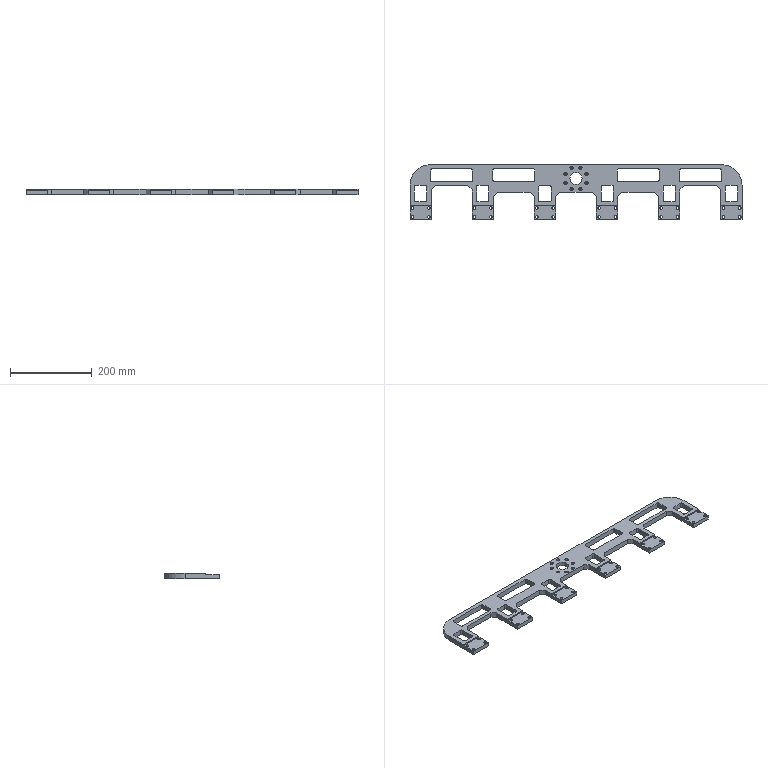NC program | NX | posted with a generic post | part box 813.6 x 134 x 13 mm
Lines 1 to 121 of 13853:
N10 G17 G21 G94 G90
(FLOOR_WALL_COPY , TOOL : D63)
N12 T01 M6
N14 G54
N16 G17 G0 G90 X-443.3 Y68.997 S6500 M3
N18 G43 Z30. H1
N20 Z3.
N22 G94 G1 Z0. F1500.
N24 X-440.3
N26 X440.3
N28 Y40.798
N30 X-440.3
N32 Y12.599
N34 X440.3
N36 Y-15.601
N38 X-440.3
N40 Y-43.8
N42 X440.3
N44 X443.3
N46 Z3.
N48 G0 Z30.
N50 M5
(DRILLING_COPY_1 , TOOL : D6A45)
N52 T07 M6
N54 G54
N56 G17 G0 G90 X-400.8 Y-61.2 S5000 M3
N58 G43 Z30. H7
N60 G94 G81 G98 Z-1. F250. R3.
N62 Y-39.2
N64 X-360.8
N66 Y-61.2
N68 X-248.4 Y-39.2
N70 Y-61.2
N72 X-208.4
N74 Y-39.2
N76 X-96.
N78 Y-61.2
N80 X-56.
N82 Y-39.2
N84 X-10.715 Y7.131
N86 X-25.869 Y22.285
N88 Y43.715
N90 X-10.715 Y58.869
N92 X10.715
N94 X25.869 Y43.715
N96 X0. Y33.
N98 X25.869 Y22.285
N100 X10.715 Y7.131
N102 X56.4 Y-39.2
N104 Y-61.2
N106 X96.4
N108 Y-39.2
N110 X208.8
N112 Y-61.2
N114 X248.8
N116 Y-39.2
N118 X361.2
N120 Y-61.2
N122 X401.2
N124 Y-39.2
N126 G80
N128 G0 X401.2 Y-39.2 Z30.
N130 M5
(DRILLING_COPY_COPY_1 , TOOL : 4.5ZT)
N132 T14 M6
N134 G54
N136 G17 G0 G90 X10.715 Y7.131 S2000 M3
N138 G43 Z30. H14
N140 G94 G83 G98 Z-15.352 F250. Q2. R3.
N142 X-10.715
N144 X-25.869 Y22.285
N146 Y43.715
N148 X-10.715 Y58.869
N150 X10.715
N152 X25.869 Y43.715
N154 Y22.285
N156 G80
N158 G0 X25.869 Y22.285 Z30.
N160 M5
(DRILLING_COPY_COPY_COPY , TOOL : 6.5ZT)
N162 T15 M6
N164 G54
N166 G17 G0 G90 X-400.8 Y-39.2 S2000 M3
N168 G43 Z30. H15
N170 G94 G83 G98 Z-15.953 F250. Q2. R3.
N172 Y-61.2
N174 X-360.8
N176 Y-39.2
N178 X-248.4
N180 Y-61.2
N182 X-208.4
N184 Y-39.2
N186 X-96.
N188 Y-61.2
N190 X-56.
N192 Y-39.2
N194 X56.4
N196 Y-61.2
N198 X96.4
N200 Y-39.2
N202 X208.8
N204 Y-61.2
N206 X248.8
N208 Y-39.2
N210 X361.2
N212 Y-61.2
N214 X401.2
N216 Y-39.2
N218 G80
N220 G0 X401.2 Y-39.2 Z30.
N222 M5